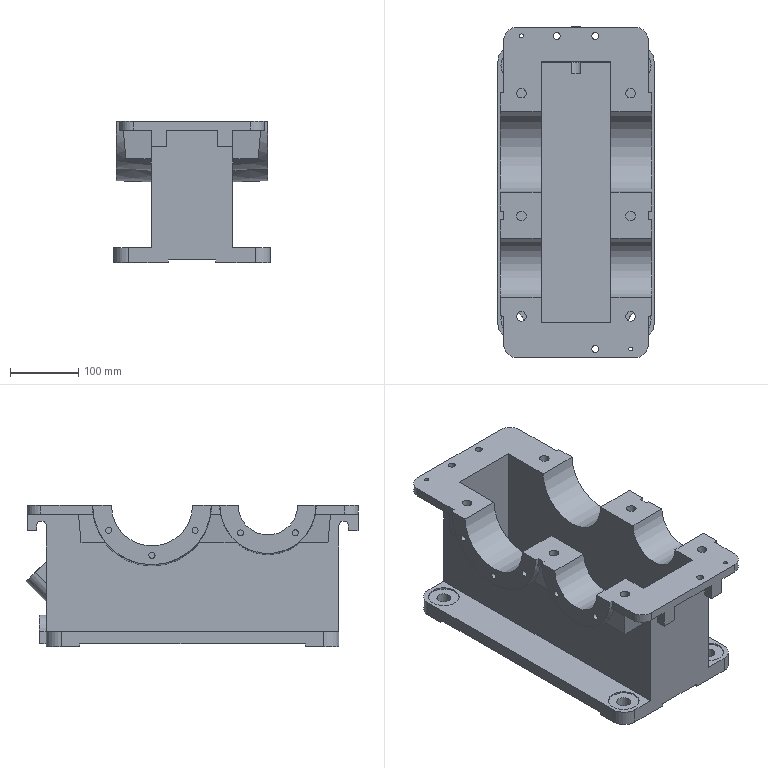Part | NX | features DATUM_CSYS 44, SKETCH 43, EXTRUDE 42, EXTRACT_DATUM_AXIS 38, EXTRACT_FACE 32, SIMPLE HOLE 25, EXTRACT_DATUM_PLANE 14, Instance Feature 13, HOLE PACKAGE 10, DRAFT 9, EXTRACT_STRING 8, FSET 6, Mirror Feature 5, BLEND 4, OFFSET_REGION 4, Pattern Feature 2 | 1 solid | 174 faces | box 229 x 486.698 x 207 mm | volume 5319663 mm3 | plane 110 | cylinder 60 | cone 4 | commonest cylinder face diameters 9 x10 14 x10 20 x7 28 x6 10 x4 40 x4